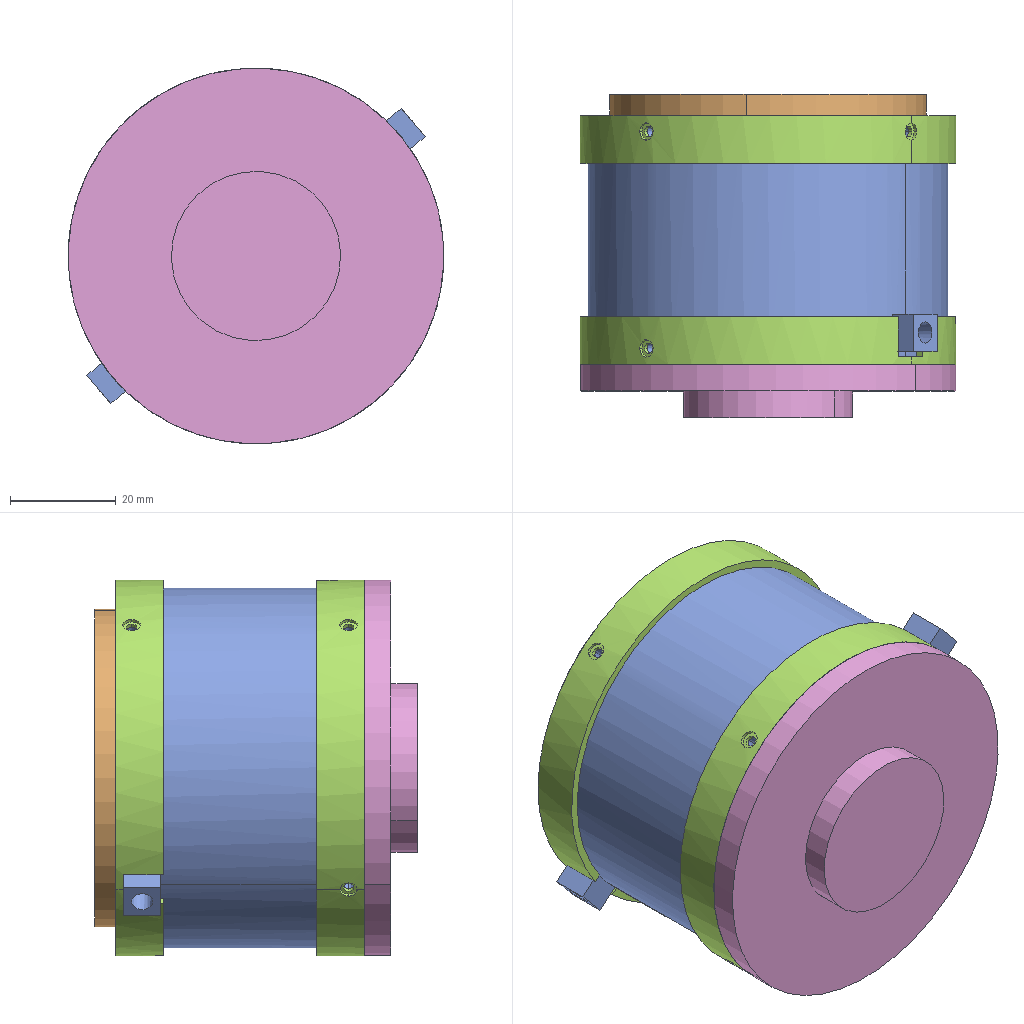Assembly | SolidWorks | 6 different items | 7 placed | box 71 x 61 x 71 mm
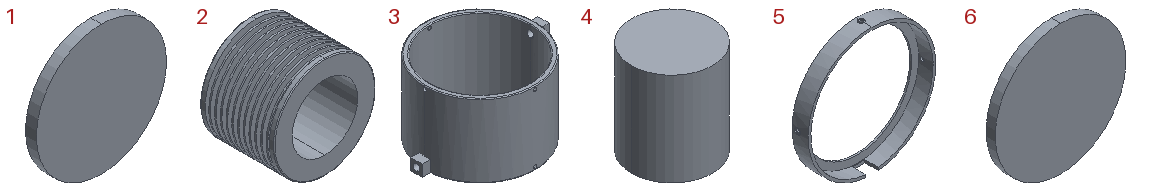Parts list (item | quantity | size | volume | features):
1 | x1 | 60 x 5 x 60 mm | 14137 mm3 | features Extrusion 1
2 | x1 | 62 x 45 x 62 mm | 37551 mm3 | features Fillet 2, Helix 1, Revolution 1, Sweep 1
3 | x1 | 78 x 68 x 45 mm | 27762 mm3 | features ICE 6, Fillet 3, CirPattern 2, Revolution 1
4 | x1 | 40 x 40 x 46 mm | 57805 mm3 | features Extrusion 1
5 | x2 | 71 x 9 x 71 mm | 3648 mm3 | features ICE 3, CirPattern 2, Revolution 1
6 | x1 | 71 x 10 x 71 mm | 23815 mm3 | features Extrusion 1, ICE 1
Mates (type | each side: item.copy, entity, surface, feature):
Concentric | 2.1 face cylinder Revolve1 | 3.1 face cylinder Revolve1
Coincident | 2.1 face plane Revolve1 | 3.1 face plane Revolve1
Concentric | 3.1 face cylinder Revolve1 | 5.1 face cylinder Revolve1
Coincident | 2.1 face plane Revolve1 | 5.1 face plane Revolve1
Concentric | 3.1 face cylinder Revolve1 | 5.2 face cylinder Revolve1
Parallel | 3.1 face plane Boss-Extrude1 | 5.2 face plane Cut-Extrude1
Coincident | 2.1 face plane Revolve1 | 5.2 face plane Revolve1
Parallel | 3.1 face plane Boss-Extrude2 | 5.1 face plane Cut-Extrude1
Coincident | 5.2 face plane Revolve1 | 6.1 face plane Boss-Extrude1
Concentric | 5.2 face cylinder Revolve1 | 6.1 face cylinder Boss-Extrude1
Concentric | 2.1 face cylinder Revolve1 | 4.1 face cylinder Boss-Extrude1
Coincident | 6.1 face plane Boss-Extrude1 | 4.1 face plane Boss-Extrude1
Coincident | 2.1 face plane Revolve1 | 1.1 face plane Boss-Extrude1
Concentric | 5.1 face cylinder Revolve1 | 1.1 face cylinder Boss-Extrude1